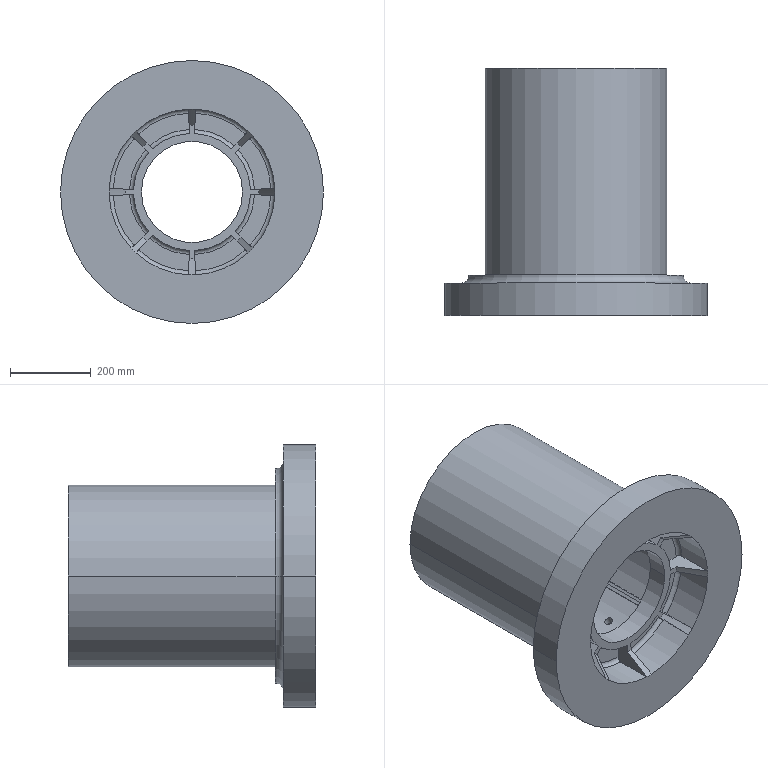Part | SolidWorks | features ICE 4, Revolution 2, CirPattern 1 | 1 solid | 128 faces | box 650 x 611.2 x 650 mm | volume 36285371 mm3 | cylinder 48 | plane 46 | torus 18 | spline 8 | cone 8 | commonest cylinder face diameters 350 x16 410 x16 290 x8 20 x2 250 x2 450 x2